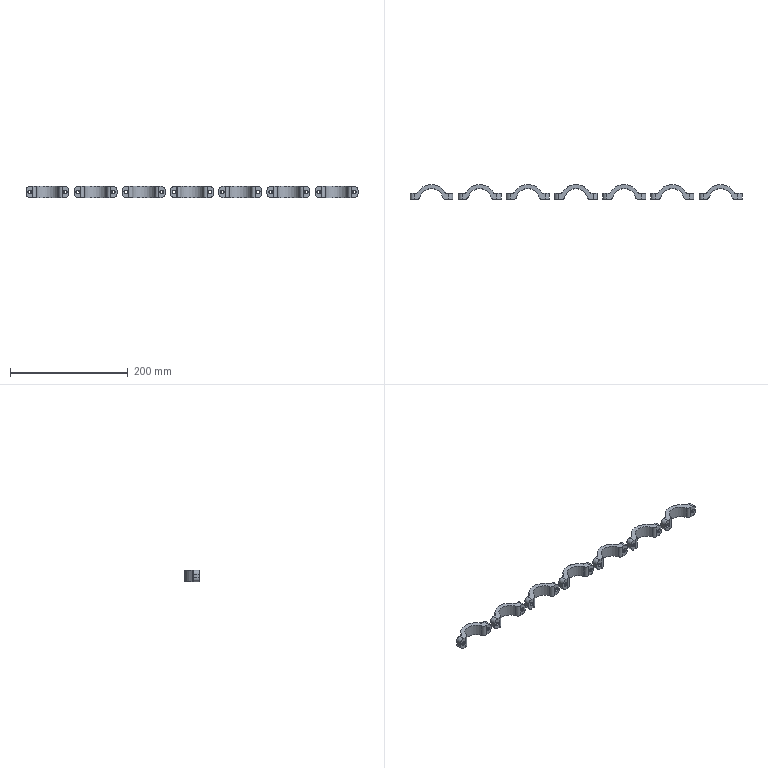NC program | Mastercam | posted with a generic post
Lines 1390 to 2922 of 23883:
(8 FI |TOOL - 2|DIA. OFF. - 2|LEN. - 2|TOOL DIA. - 8.)
N2848 T2 M6
N2850 G0 G56 G90 X28.858 Y7.56 C0. B0. S3500 M3
N2852 G43 H2 Z50.
N2854 Z1.
N2856 G1 Z-.5 F2000.
N2858 G41 D2 X24.866 Y4.549 F800.
N2860 G3 X24.786 Y4.389 I.121 J-.16
N2862 X24.827 Y4.269 I.201
N2864 G2 X26.441 Y1.912 I-24.827 J-18.731
N2866 G3 X26.714 Y1.475 I5.579 J3.182
N2868 X27.143 Y1.461 I.429 J6.407
N2870 X27.255 Y1.462 J6.421
N2872 G1 X31.884
N2874 G3 X32.084 Y1.662 J.2
N2876 G1 G40 Y6.662
N2878 X28.858 Y7.56
N2880 Z-1. F2000.
N2882 G41 D2 X24.866 Y4.549 F800.
N2884 G3 X24.786 Y4.389 I.121 J-.16
N2886 X24.827 Y4.269 I.201
N2888 G2 X26.441 Y1.912 I-24.827 J-18.731
N2890 G3 X26.714 Y1.475 I5.579 J3.182
N2892 X27.143 Y1.461 I.429 J6.407
N2894 X27.255 Y1.462 J6.421
N2896 G1 X31.884
N2898 G3 X32.084 Y1.662 J.2
N2900 G1 G40 Y6.662
N2902 X28.858 Y7.56
N2904 Z-1.5 F2000.
N2906 G41 D2 X24.866 Y4.549 F800.
N2908 G3 X24.786 Y4.389 I.121 J-.16
N2910 X24.827 Y4.269 I.201
N2912 G2 X26.441 Y1.912 I-24.827 J-18.731
N2914 G3 X26.714 Y1.475 I5.579 J3.182
N2916 X27.143 Y1.461 I.429 J6.407
N2918 X27.255 Y1.462 J6.421
N2920 G1 X31.884
N2922 G3 X32.084 Y1.662 J.2
N2924 G1 G40 Y6.662
N2926 X28.858 Y7.56
N2928 Z-2. F2000.
N2930 G41 D2 X24.866 Y4.549 F800.
N2932 G3 X24.786 Y4.389 I.121 J-.16
N2934 X24.827 Y4.269 I.201
N2936 G2 X26.441 Y1.912 I-24.827 J-18.731
N2938 G3 X26.714 Y1.475 I5.579 J3.182
N2940 X27.143 Y1.461 I.429 J6.407
N2942 X27.255 Y1.462 J6.421
N2944 G1 X31.884
N2946 G3 X32.084 Y1.662 J.2
N2948 G1 G40 Y6.662
N2950 X28.858 Y7.56
N2952 Z-2.5 F2000.
N2954 G41 D2 X24.866 Y4.549 F800.
N2956 G3 X24.786 Y4.389 I.121 J-.16
N2958 X24.827 Y4.269 I.201
N2960 G2 X26.441 Y1.912 I-24.827 J-18.731
N2962 G3 X26.714 Y1.475 I5.579 J3.182
N2964 X27.143 Y1.461 I.429 J6.407
N2966 X27.255 Y1.462 J6.421
N2968 G1 X31.884
N2970 G3 X32.084 Y1.662 J.2
N2972 G1 G40 Y6.662
N2974 X28.858 Y7.56
N2976 Z-3. F2000.
N2978 G41 D2 X24.866 Y4.549 F800.
N2980 G3 X24.786 Y4.389 I.121 J-.16
N2982 X24.827 Y4.269 I.201
N2984 G2 X26.441 Y1.912 I-24.827 J-18.731
N2986 G3 X26.714 Y1.475 I5.579 J3.182
N2988 X27.143 Y1.461 I.429 J6.407
N2990 X27.255 Y1.462 J6.421
N2992 G1 X31.884
N2994 G3 X32.084 Y1.662 J.2
N2996 G1 G40 Y6.662
N2998 X28.858 Y7.56
N3000 Z-3.5 F2000.
N3002 G41 D2 X24.866 Y4.549 F800.
N3004 G3 X24.786 Y4.389 I.121 J-.16
N3006 X24.827 Y4.269 I.201
N3008 G2 X26.441 Y1.912 I-24.827 J-18.731
N3010 G3 X26.714 Y1.475 I5.579 J3.182
N3012 X27.143 Y1.461 I.429 J6.407
N3014 X27.255 Y1.462 J6.421
N3016 G1 X31.884
N3018 G3 X32.084 Y1.662 J.2
N3020 G1 G40 Y6.662
N3022 X28.858 Y7.56
N3024 Z-4. F2000.
N3026 G41 D2 X24.866 Y4.549 F800.
N3028 G3 X24.786 Y4.389 I.121 J-.16
N3030 X24.827 Y4.269 I.201
N3032 G2 X26.441 Y1.912 I-24.827 J-18.731
N3034 G3 X26.714 Y1.475 I5.579 J3.182
N3036 X27.143 Y1.461 I.429 J6.407
N3038 X27.255 Y1.462 J6.421
N3040 G1 X31.884
N3042 G3 X32.084 Y1.662 J.2
N3044 G1 G40 Y6.662
N3046 X28.858 Y7.56
N3048 Z-4.5 F2000.
N3050 G41 D2 X24.866 Y4.549 F800.
N3052 G3 X24.786 Y4.389 I.121 J-.16
N3054 X24.827 Y4.269 I.201
N3056 G2 X26.441 Y1.912 I-24.827 J-18.731
N3058 G3 X26.714 Y1.475 I5.579 J3.182
N3060 X27.143 Y1.461 I.429 J6.407
N3062 X27.255 Y1.462 J6.421
N3064 G1 X31.884
N3066 G3 X32.084 Y1.662 J.2
N3068 G1 G40 Y6.662
N3070 X28.858 Y7.56
N3072 Z-5. F2000.
N3074 G41 D2 X24.866 Y4.549 F800.
N3076 G3 X24.786 Y4.389 I.121 J-.16
N3078 X24.827 Y4.269 I.201
N3080 G2 X26.441 Y1.912 I-24.827 J-18.731
N3082 G3 X26.714 Y1.475 I5.579 J3.182
N3084 X27.143 Y1.461 I.429 J6.407
N3086 X27.255 Y1.462 J6.421
N3088 G1 X31.884
N3090 G3 X32.084 Y1.662 J.2
N3092 G1 G40 Y6.662
N3094 X28.858 Y7.56
N3096 Z-5.5 F2000.
N3098 G41 D2 X24.866 Y4.549 F800.
N3100 G3 X24.786 Y4.389 I.121 J-.16
N3102 X24.827 Y4.269 I.201
N3104 G2 X26.441 Y1.912 I-24.827 J-18.731
N3106 G3 X26.714 Y1.475 I5.579 J3.182
N3108 X27.143 Y1.461 I.429 J6.407
N3110 X27.255 Y1.462 J6.421
N3112 G1 X31.884
N3114 G3 X32.084 Y1.662 J.2
N3116 G1 G40 Y6.662
N3118 X28.858 Y7.56
N3120 Z-6. F2000.
N3122 G41 D2 X24.866 Y4.549 F800.
N3124 G3 X24.786 Y4.389 I.121 J-.16
N3126 X24.827 Y4.269 I.201
N3128 G2 X26.441 Y1.912 I-24.827 J-18.731
N3130 G3 X26.714 Y1.475 I5.579 J3.182
N3132 X27.143 Y1.461 I.429 J6.407
N3134 X27.255 Y1.462 J6.421
N3136 G1 X31.884
N3138 G3 X32.084 Y1.662 J.2
N3140 G1 G40 Y6.662
N3142 X28.858 Y7.56
N3144 Z-6.5 F2000.
N3146 G41 D2 X24.866 Y4.549 F800.
N3148 G3 X24.786 Y4.389 I.121 J-.16
N3150 X24.827 Y4.269 I.201
N3152 G2 X26.441 Y1.912 I-24.827 J-18.731
N3154 G3 X26.714 Y1.475 I5.579 J3.182
N3156 X27.143 Y1.461 I.429 J6.407
N3158 X27.255 Y1.462 J6.421
N3160 G1 X31.884
N3162 G3 X32.084 Y1.662 J.2
N3164 G1 G40 Y6.662
N3166 X28.858 Y7.56
N3168 Z-7. F2000.
N3170 G41 D2 X24.866 Y4.549 F800.
N3172 G3 X24.786 Y4.389 I.121 J-.16
N3174 X24.827 Y4.269 I.201
N3176 G2 X26.441 Y1.912 I-24.827 J-18.731
N3178 G3 X26.714 Y1.475 I5.579 J3.182
N3180 X27.143 Y1.461 I.429 J6.407
N3182 X27.255 Y1.462 J6.421
N3184 G1 X31.884
N3186 G3 X32.084 Y1.662 J.2
N3188 G1 G40 Y6.662
N3190 X28.858 Y7.56
N3192 Z-7.5 F2000.
N3194 G41 D2 X24.866 Y4.549 F800.
N3196 G3 X24.786 Y4.389 I.121 J-.16
N3198 X24.827 Y4.269 I.201
N3200 G2 X26.441 Y1.912 I-24.827 J-18.731
N3202 G3 X26.714 Y1.475 I5.579 J3.182
N3204 X27.143 Y1.461 I.429 J6.407
N3206 X27.255 Y1.462 J6.421
N3208 G1 X31.884
N3210 G3 X32.084 Y1.662 J.2
N3212 G1 G40 Y6.662
N3214 X28.858 Y7.56
N3216 Z-8. F2000.
N3218 G41 D2 X24.866 Y4.549 F800.
N3220 G3 X24.786 Y4.389 I.121 J-.16
N3222 X24.827 Y4.269 I.201
N3224 G2 X26.441 Y1.912 I-24.827 J-18.731
N3226 G3 X26.714 Y1.475 I5.579 J3.182
N3228 X27.143 Y1.461 I.429 J6.407
N3230 X27.255 Y1.462 J6.421
N3232 G1 X31.884
N3234 G3 X32.084 Y1.662 J.2
N3236 G1 G40 Y6.662
N3238 X28.858 Y7.56
N3240 Z-8.5 F2000.
N3242 G41 D2 X24.866 Y4.549 F800.
N3244 G3 X24.786 Y4.389 I.121 J-.16
N3246 X24.827 Y4.269 I.201
N3248 G2 X26.441 Y1.912 I-24.827 J-18.731
N3250 G3 X26.714 Y1.475 I5.579 J3.182
N3252 X27.143 Y1.461 I.429 J6.407
N3254 X27.255 Y1.462 J6.421
N3256 G1 X31.884
N3258 G3 X32.084 Y1.662 J.2
N3260 G1 G40 Y6.662
N3262 X28.858 Y7.56
N3264 Z-9. F2000.
N3266 G41 D2 X24.866 Y4.549 F800.
N3268 G3 X24.786 Y4.389 I.121 J-.16
N3270 X24.827 Y4.269 I.201
N3272 G2 X26.441 Y1.912 I-24.827 J-18.731
N3274 G3 X26.714 Y1.475 I5.579 J3.182
N3276 X27.143 Y1.461 I.429 J6.407
N3278 X27.255 Y1.462 J6.421
N3280 G1 X31.884
N3282 G3 X32.084 Y1.662 J.2
N3284 G1 G40 Y6.662
N3286 X28.858 Y7.56
N3288 Z-9.5 F2000.
N3290 G41 D2 X24.866 Y4.549 F800.
N3292 G3 X24.786 Y4.389 I.121 J-.16
N3294 X24.827 Y4.269 I.201
N3296 G2 X26.441 Y1.912 I-24.827 J-18.731
N3298 G3 X26.714 Y1.475 I5.579 J3.182
N3300 X27.143 Y1.461 I.429 J6.407
N3302 X27.255 Y1.462 J6.421
N3304 G1 X31.884
N3306 G3 X32.084 Y1.662 J.2
N3308 G1 G40 Y6.662
N3310 X28.858 Y7.56
N3312 Z-10. F2000.
N3314 G41 D2 X24.866 Y4.549 F800.
N3316 G3 X24.786 Y4.389 I.121 J-.16
N3318 X24.827 Y4.269 I.201
N3320 G2 X26.441 Y1.912 I-24.827 J-18.731
N3322 G3 X26.714 Y1.475 I5.579 J3.182
N3324 X27.143 Y1.461 I.429 J6.407
N3326 X27.255 Y1.462 J6.421
N3328 G1 X31.884
N3330 G3 X32.084 Y1.662 J.2
N3332 G1 G40 Y6.662
N3334 X28.858 Y7.56
N3336 Z-10.5 F2000.
N3338 G41 D2 X24.866 Y4.549 F800.
N3340 G3 X24.786 Y4.389 I.121 J-.16
N3342 X24.827 Y4.269 I.201
N3344 G2 X26.441 Y1.912 I-24.827 J-18.731
N3346 G3 X26.714 Y1.475 I5.579 J3.182
N3348 X27.143 Y1.461 I.429 J6.407
N3350 X27.255 Y1.462 J6.421
N3352 G1 X31.884
N3354 G3 X32.084 Y1.662 J.2
N3356 G1 G40 Y6.662
N3358 X28.858 Y7.56
N3360 Z-11. F2000.
N3362 G41 D2 X24.866 Y4.549 F800.
N3364 G3 X24.786 Y4.389 I.121 J-.16
N3366 X24.827 Y4.269 I.201
N3368 G2 X26.441 Y1.912 I-24.827 J-18.731
N3370 G3 X26.714 Y1.475 I5.579 J3.182
N3372 X27.143 Y1.461 I.429 J6.407
N3374 X27.255 Y1.462 J6.421
N3376 G1 X31.884
N3378 G3 X32.084 Y1.662 J.2
N3380 G1 G40 Y6.662
N3382 X28.858 Y7.56
N3384 Z-11.5 F2000.
N3386 G41 D2 X24.866 Y4.549 F800.
N3388 G3 X24.786 Y4.389 I.121 J-.16
N3390 X24.827 Y4.269 I.201
N3392 G2 X26.441 Y1.912 I-24.827 J-18.731
N3394 G3 X26.714 Y1.475 I5.579 J3.182
N3396 X27.143 Y1.461 I.429 J6.407
N3398 X27.255 Y1.462 J6.421
N3400 G1 X31.884
N3402 G3 X32.084 Y1.662 J.2
N3404 G1 G40 Y6.662
N3406 X28.858 Y7.56
N3408 Z-12. F2000.
N3410 G41 D2 X24.866 Y4.549 F800.
N3412 G3 X24.786 Y4.389 I.121 J-.16
N3414 X24.827 Y4.269 I.201
N3416 G2 X26.441 Y1.912 I-24.827 J-18.731
N3418 G3 X26.714 Y1.475 I5.579 J3.182
N3420 X27.143 Y1.461 I.429 J6.407
N3422 X27.255 Y1.462 J6.421
N3424 G1 X31.884
N3426 G3 X32.084 Y1.662 J.2
N3428 G1 G40 Y6.662
N3430 X28.858 Y7.56
N3432 Z-12.5 F2000.
N3434 G41 D2 X24.866 Y4.549 F800.
N3436 G3 X24.786 Y4.389 I.121 J-.16
N3438 X24.827 Y4.269 I.201
N3440 G2 X26.441 Y1.912 I-24.827 J-18.731
N3442 G3 X26.714 Y1.475 I5.579 J3.182
N3444 X27.143 Y1.461 I.429 J6.407
N3446 X27.255 Y1.462 J6.421
N3448 G1 X31.884
N3450 G3 X32.084 Y1.662 J.2
N3452 G1 G40 Y6.662
N3454 X28.858 Y7.56
N3456 Z-13. F2000.
N3458 G41 D2 X24.866 Y4.549 F800.
N3460 G3 X24.786 Y4.389 I.121 J-.16
N3462 X24.827 Y4.269 I.201
N3464 G2 X26.441 Y1.912 I-24.827 J-18.731
N3466 G3 X26.714 Y1.475 I5.579 J3.182
N3468 X27.143 Y1.461 I.429 J6.407
N3470 X27.255 Y1.462 J6.421
N3472 G1 X31.884
N3474 G3 X32.084 Y1.662 J.2
N3476 G1 G40 Y6.662
N3478 X28.858 Y7.56
N3480 Z-13.5 F2000.
N3482 G41 D2 X24.866 Y4.549 F800.
N3484 G3 X24.786 Y4.389 I.121 J-.16
N3486 X24.827 Y4.269 I.201
N3488 G2 X26.441 Y1.912 I-24.827 J-18.731
N3490 G3 X26.714 Y1.475 I5.579 J3.182
N3492 X27.143 Y1.461 I.429 J6.407
N3494 X27.255 Y1.462 J6.421
N3496 G1 X31.884
N3498 G3 X32.084 Y1.662 J.2
N3500 G1 G40 Y6.662
N3502 X28.858 Y7.56
N3504 Z-14. F2000.
N3506 G41 D2 X24.866 Y4.549 F800.
N3508 G3 X24.786 Y4.389 I.121 J-.16
N3510 X24.827 Y4.269 I.201
N3512 G2 X26.441 Y1.912 I-24.827 J-18.731
N3514 G3 X26.714 Y1.475 I5.579 J3.182
N3516 X27.143 Y1.461 I.429 J6.407
N3518 X27.255 Y1.462 J6.421
N3520 G1 X31.884
N3522 G3 X32.084 Y1.662 J.2
N3524 G1 G40 Y6.662
N3526 X28.858 Y7.56
N3528 Z-14.5 F2000.
N3530 G41 D2 X24.866 Y4.549 F800.
N3532 G3 X24.786 Y4.389 I.121 J-.16
N3534 X24.827 Y4.269 I.201
N3536 G2 X26.441 Y1.912 I-24.827 J-18.731
N3538 G3 X26.714 Y1.475 I5.579 J3.182
N3540 X27.143 Y1.461 I.429 J6.407
N3542 X27.255 Y1.462 J6.421
N3544 G1 X31.884
N3546 G3 X32.084 Y1.662 J.2
N3548 G1 G40 Y6.662
N3550 X28.858 Y7.56
N3552 Z-15. F2000.
N3554 G41 D2 X24.866 Y4.549 F800.
N3556 G3 X24.786 Y4.389 I.121 J-.16
N3558 X24.827 Y4.269 I.201
N3560 G2 X26.441 Y1.912 I-24.827 J-18.731
N3562 G3 X26.714 Y1.475 I5.579 J3.182
N3564 X27.143 Y1.461 I.429 J6.407
N3566 X27.255 Y1.462 J6.421
N3568 G1 X31.884
N3570 G3 X32.084 Y1.662 J.2
N3572 G1 G40 Y6.662
N3574 X28.858 Y7.56
N3576 Z-15.5 F2000.
N3578 G41 D2 X24.866 Y4.549 F800.
N3580 G3 X24.786 Y4.389 I.121 J-.16
N3582 X24.827 Y4.269 I.201
N3584 G2 X26.441 Y1.912 I-24.827 J-18.731
N3586 G3 X26.714 Y1.475 I5.579 J3.182
N3588 X27.143 Y1.461 I.429 J6.407
N3590 X27.255 Y1.462 J6.421
N3592 G1 X31.884
N3594 G3 X32.084 Y1.662 J.2
N3596 G1 G40 Y6.662
N3598 X28.858 Y7.56
N3600 Z-16. F2000.
N3602 G41 D2 X24.866 Y4.549 F800.
N3604 G3 X24.786 Y4.389 I.121 J-.16
N3606 X24.827 Y4.269 I.201
N3608 G2 X26.441 Y1.912 I-24.827 J-18.731
N3610 G3 X26.714 Y1.475 I5.579 J3.182
N3612 X27.143 Y1.461 I.429 J6.407
N3614 X27.255 Y1.462 J6.421
N3616 G1 X31.884
N3618 G3 X32.084 Y1.662 J.2
N3620 G1 G40 Y6.662
N3622 X28.858 Y7.56
N3624 Z-16.5 F2000.
N3626 G41 D2 X24.866 Y4.549 F800.
N3628 G3 X24.786 Y4.389 I.121 J-.16
N3630 X24.827 Y4.269 I.201
N3632 G2 X26.441 Y1.912 I-24.827 J-18.731
N3634 G3 X26.714 Y1.475 I5.579 J3.182
N3636 X27.143 Y1.461 I.429 J6.407
N3638 X27.255 Y1.462 J6.421
N3640 G1 X31.884
N3642 G3 X32.084 Y1.662 J.2
N3644 G1 G40 Y6.662
N3646 X28.858 Y7.56
N3648 Z-17. F2000.
N3650 G41 D2 X24.866 Y4.549 F800.
N3652 G3 X24.786 Y4.389 I.121 J-.16
N3654 X24.827 Y4.269 I.201
N3656 G2 X26.441 Y1.912 I-24.827 J-18.731
N3658 G3 X26.714 Y1.475 I5.579 J3.182
N3660 X27.143 Y1.461 I.429 J6.407
N3662 X27.255 Y1.462 J6.421
N3664 G1 X31.884
N3666 G3 X32.084 Y1.662 J.2
N3668 G1 G40 Y6.662
N3670 X28.858 Y7.56
N3672 Z-17.5 F2000.
N3674 G41 D2 X24.866 Y4.549 F800.
N3676 G3 X24.786 Y4.389 I.121 J-.16
N3678 X24.827 Y4.269 I.201
N3680 G2 X26.441 Y1.912 I-24.827 J-18.731
N3682 G3 X26.714 Y1.475 I5.579 J3.182
N3684 X27.143 Y1.461 I.429 J6.407
N3686 X27.255 Y1.462 J6.421
N3688 G1 X31.884
N3690 G3 X32.084 Y1.662 J.2
N3692 G1 G40 Y6.662
N3694 X28.858 Y7.56
N3696 Z-18. F2000.
N3698 G41 D2 X24.866 Y4.549 F800.
N3700 G3 X24.786 Y4.389 I.121 J-.16
N3702 X24.827 Y4.269 I.201
N3704 G2 X26.441 Y1.912 I-24.827 J-18.731
N3706 G3 X26.714 Y1.475 I5.579 J3.182
N3708 X27.143 Y1.461 I.429 J6.407
N3710 X27.255 Y1.462 J6.421
N3712 G1 X31.884
N3714 G3 X32.084 Y1.662 J.2
N3716 G1 G40 Y6.662
N3718 X28.858 Y7.56
N3720 Z-18.5 F2000.
N3722 G41 D2 X24.866 Y4.549 F800.
N3724 G3 X24.786 Y4.389 I.121 J-.16
N3726 X24.827 Y4.269 I.201
N3728 G2 X26.441 Y1.912 I-24.827 J-18.731
N3730 G3 X26.714 Y1.475 I5.579 J3.182
N3732 X27.143 Y1.461 I.429 J6.407
N3734 X27.255 Y1.462 J6.421
N3736 G1 X31.884
N3738 G3 X32.084 Y1.662 J.2
N3740 G1 G40 Y6.662
N3742 X28.858 Y7.56
N3744 Z-19. F2000.
N3746 G41 D2 X24.866 Y4.549 F800.
N3748 G3 X24.786 Y4.389 I.121 J-.16
N3750 X24.827 Y4.269 I.201
N3752 G2 X26.441 Y1.912 I-24.827 J-18.731
N3754 G3 X26.714 Y1.475 I5.579 J3.182
N3756 X27.143 Y1.461 I.429 J6.407
N3758 X27.255 Y1.462 J6.421
N3760 G1 X31.884
N3762 G3 X32.084 Y1.662 J.2
N3764 G1 G40 Y6.662
N3766 X28.858 Y7.56
N3768 Z-19.5 F2000.
N3770 G41 D2 X24.866 Y4.549 F800.
N3772 G3 X24.786 Y4.389 I.121 J-.16
N3774 X24.827 Y4.269 I.201
N3776 G2 X26.441 Y1.912 I-24.827 J-18.731
N3778 G3 X26.714 Y1.475 I5.579 J3.182
N3780 X27.143 Y1.461 I.429 J6.407
N3782 X27.255 Y1.462 J6.421
N3784 G1 X31.884
N3786 G3 X32.084 Y1.662 J.2
N3788 G1 G40 Y6.662
N3790 X28.858 Y7.56
N3792 Z-20. F2000.
N3794 G41 D2 X24.866 Y4.549 F800.
N3796 G3 X24.786 Y4.389 I.121 J-.16
N3798 X24.827 Y4.269 I.201
N3800 G2 X26.441 Y1.912 I-24.827 J-18.731
N3802 G3 X26.714 Y1.475 I5.579 J3.182
N3804 X27.143 Y1.461 I.429 J6.407
N3806 X27.255 Y1.462 J6.421
N3808 G1 X31.884
N3810 G3 X32.084 Y1.662 J.2
N3812 G1 G40 Y6.662
N3814 X28.858 Y7.56
N3816 Z-20.5 F2000.
N3818 G41 D2 X24.866 Y4.549 F800.
N3820 G3 X24.786 Y4.389 I.121 J-.16
N3822 X24.827 Y4.269 I.201
N3824 G2 X26.441 Y1.912 I-24.827 J-18.731
N3826 G3 X26.714 Y1.475 I5.579 J3.182
N3828 X27.143 Y1.461 I.429 J6.407
N3830 X27.255 Y1.462 J6.421
N3832 G1 X31.884
N3834 G3 X32.084 Y1.662 J.2
N3836 G1 G40 Y6.662
N3838 X28.858 Y7.56
N3840 Z-21. F2000.
N3842 G41 D2 X24.866 Y4.549 F800.
N3844 G3 X24.786 Y4.389 I.121 J-.16
N3846 X24.827 Y4.269 I.201
N3848 G2 X26.441 Y1.912 I-24.827 J-18.731
N3850 G3 X26.714 Y1.475 I5.579 J3.182
N3852 X27.143 Y1.461 I.429 J6.407
N3854 X27.255 Y1.462 J6.421
N3856 G1 X31.884
N3858 G3 X32.084 Y1.662 J.2
N3860 G1 G40 Y6.662
N3862 G0 Z50.
N3864 X-32.052
N3866 Z1.
N3868 G1 Z-.5 F2000.
N3870 G41 D2 Y1.662 F800.
N3872 G3 X-31.852 Y1.462 I.2
N3874 G1 X-27.264
N3876 X-26.719 Y1.47
N3878 G2 X-24.827 Y4.269 I28.979 J-17.547
N3880 G3 X-24.787 Y4.389 I-.16 J.12
N3882 X-24.866 Y4.549 I-.2
N3884 G1 G40 X-28.858 Y7.56
N3886 X-32.052 Y6.662
N3888 Z-1. F2000.
N3890 G41 D2 Y1.662 F800.
N3892 G3 X-31.852 Y1.462 I.2
N3894 G1 X-27.264
N3896 X-26.719 Y1.47
N3898 G2 X-24.827 Y4.269 I28.979 J-17.547
N3900 G3 X-24.787 Y4.389 I-.16 J.12
N3902 X-24.866 Y4.549 I-.2
N3904 G1 G40 X-28.858 Y7.56
N3906 X-32.052 Y6.662
N3908 Z-1.5 F2000.
N3910 G41 D2 Y1.662 F800.
N3912 G3 X-31.852 Y1.462 I.2
N3914 G1 X-27.264
N3916 X-26.719 Y1.47
N3918 G2 X-24.827 Y4.269 I28.979 J-17.547
N3920 G3 X-24.787 Y4.389 I-.16 J.12
N3922 X-24.866 Y4.549 I-.2
N3924 G1 G40 X-28.858 Y7.56
N3926 X-32.052 Y6.662
N3928 Z-2. F2000.
N3930 G41 D2 Y1.662 F800.
N3932 G3 X-31.852 Y1.462 I.2
N3934 G1 X-27.264
N3936 X-26.719 Y1.47
N3938 G2 X-24.827 Y4.269 I28.979 J-17.547
N3940 G3 X-24.787 Y4.389 I-.16 J.12
N3942 X-24.866 Y4.549 I-.2
N3944 G1 G40 X-28.858 Y7.56
N3946 X-32.052 Y6.662
N3948 Z-2.5 F2000.
N3950 G41 D2 Y1.662 F800.
N3952 G3 X-31.852 Y1.462 I.2
N3954 G1 X-27.264
N3956 X-26.719 Y1.47
N3958 G2 X-24.827 Y4.269 I28.979 J-17.547
N3960 G3 X-24.787 Y4.389 I-.16 J.12
N3962 X-24.866 Y4.549 I-.2
N3964 G1 G40 X-28.858 Y7.56
N3966 X-32.052 Y6.662
N3968 Z-3. F2000.
N3970 G41 D2 Y1.662 F800.
N3972 G3 X-31.852 Y1.462 I.2
N3974 G1 X-27.264
N3976 X-26.719 Y1.47
N3978 G2 X-24.827 Y4.269 I28.979 J-17.547
N3980 G3 X-24.787 Y4.389 I-.16 J.12
N3982 X-24.866 Y4.549 I-.2
N3984 G1 G40 X-28.858 Y7.56
N3986 X-32.052 Y6.662
N3988 Z-3.5 F2000.
N3990 G41 D2 Y1.662 F800.
N3992 G3 X-31.852 Y1.462 I.2
N3994 G1 X-27.264
N3996 X-26.719 Y1.47
N3998 G2 X-24.827 Y4.269 I28.979 J-17.547
N4000 G3 X-24.787 Y4.389 I-.16 J.12
N4002 X-24.866 Y4.549 I-.2
N4004 G1 G40 X-28.858 Y7.56
N4006 X-32.052 Y6.662
N4008 Z-4. F2000.
N4010 G41 D2 Y1.662 F800.
N4012 G3 X-31.852 Y1.462 I.2
N4014 G1 X-27.264
N4016 X-26.719 Y1.47
N4018 G2 X-24.827 Y4.269 I28.979 J-17.547
N4020 G3 X-24.787 Y4.389 I-.16 J.12
N4022 X-24.866 Y4.549 I-.2
N4024 G1 G40 X-28.858 Y7.56
N4026 X-32.052 Y6.662
N4028 Z-4.5 F2000.
N4030 G41 D2 Y1.662 F800.
N4032 G3 X-31.852 Y1.462 I.2
N4034 G1 X-27.264
N4036 X-26.719 Y1.47
N4038 G2 X-24.827 Y4.269 I28.979 J-17.547
N4040 G3 X-24.787 Y4.389 I-.16 J.12
N4042 X-24.866 Y4.549 I-.2
N4044 G1 G40 X-28.858 Y7.56
N4046 X-32.052 Y6.662
N4048 Z-5. F2000.
N4050 G41 D2 Y1.662 F800.
N4052 G3 X-31.852 Y1.462 I.2
N4054 G1 X-27.264
N4056 X-26.719 Y1.47
N4058 G2 X-24.827 Y4.269 I28.979 J-17.547
N4060 G3 X-24.787 Y4.389 I-.16 J.12
N4062 X-24.866 Y4.549 I-.2
N4064 G1 G40 X-28.858 Y7.56
N4066 X-32.052 Y6.662
N4068 Z-5.5 F2000.
N4070 G41 D2 Y1.662 F800.
N4072 G3 X-31.852 Y1.462 I.2
N4074 G1 X-27.264
N4076 X-26.719 Y1.47
N4078 G2 X-24.827 Y4.269 I28.979 J-17.547
N4080 G3 X-24.787 Y4.389 I-.16 J.12
N4082 X-24.866 Y4.549 I-.2
N4084 G1 G40 X-28.858 Y7.56
N4086 X-32.052 Y6.662
N4088 Z-6. F2000.
N4090 G41 D2 Y1.662 F800.
N4092 G3 X-31.852 Y1.462 I.2
N4094 G1 X-27.264
N4096 X-26.719 Y1.47
N4098 G2 X-24.827 Y4.269 I28.979 J-17.547
N4100 G3 X-24.787 Y4.389 I-.16 J.12
N4102 X-24.866 Y4.549 I-.2
N4104 G1 G40 X-28.858 Y7.56
N4106 X-32.052 Y6.662
N4108 Z-6.5 F2000.
N4110 G41 D2 Y1.662 F800.
N4112 G3 X-31.852 Y1.462 I.2
N4114 G1 X-27.264
N4116 X-26.719 Y1.47
N4118 G2 X-24.827 Y4.269 I28.979 J-17.547
N4120 G3 X-24.787 Y4.389 I-.16 J.12
N4122 X-24.866 Y4.549 I-.2
N4124 G1 G40 X-28.858 Y7.56
N4126 X-32.052 Y6.662
N4128 Z-7. F2000.
N4130 G41 D2 Y1.662 F800.
N4132 G3 X-31.852 Y1.462 I.2
N4134 G1 X-27.264
N4136 X-26.719 Y1.47
N4138 G2 X-24.827 Y4.269 I28.979 J-17.547
N4140 G3 X-24.787 Y4.389 I-.16 J.12
N4142 X-24.866 Y4.549 I-.2
N4144 G1 G40 X-28.858 Y7.56
N4146 X-32.052 Y6.662
N4148 Z-7.5 F2000.
N4150 G41 D2 Y1.662 F800.
N4152 G3 X-31.852 Y1.462 I.2
N4154 G1 X-27.264
N4156 X-26.719 Y1.47
N4158 G2 X-24.827 Y4.269 I28.979 J-17.547
N4160 G3 X-24.787 Y4.389 I-.16 J.12
N4162 X-24.866 Y4.549 I-.2
N4164 G1 G40 X-28.858 Y7.56
N4166 X-32.052 Y6.662
N4168 Z-8. F2000.
N4170 G41 D2 Y1.662 F800.
N4172 G3 X-31.852 Y1.462 I.2
N4174 G1 X-27.264
N4176 X-26.719 Y1.47
N4178 G2 X-24.827 Y4.269 I28.979 J-17.547
N4180 G3 X-24.787 Y4.389 I-.16 J.12
N4182 X-24.866 Y4.549 I-.2
N4184 G1 G40 X-28.858 Y7.56
N4186 X-32.052 Y6.662
N4188 Z-8.5 F2000.
N4190 G41 D2 Y1.662 F800.
N4192 G3 X-31.852 Y1.462 I.2
N4194 G1 X-27.264
N4196 X-26.719 Y1.47
N4198 G2 X-24.827 Y4.269 I28.979 J-17.547
N4200 G3 X-24.787 Y4.389 I-.16 J.12
N4202 X-24.866 Y4.549 I-.2
N4204 G1 G40 X-28.858 Y7.56
N4206 X-32.052 Y6.662
N4208 Z-9. F2000.
N4210 G41 D2 Y1.662 F800.
N4212 G3 X-31.852 Y1.462 I.2
N4214 G1 X-27.264
N4216 X-26.719 Y1.47
N4218 G2 X-24.827 Y4.269 I28.979 J-17.547
N4220 G3 X-24.787 Y4.389 I-.16 J.12
N4222 X-24.866 Y4.549 I-.2
N4224 G1 G40 X-28.858 Y7.56
N4226 X-32.052 Y6.662
N4228 Z-9.5 F2000.
N4230 G41 D2 Y1.662 F800.
N4232 G3 X-31.852 Y1.462 I.2
N4234 G1 X-27.264
N4236 X-26.719 Y1.47
N4238 G2 X-24.827 Y4.269 I28.979 J-17.547
N4240 G3 X-24.787 Y4.389 I-.16 J.12
N4242 X-24.866 Y4.549 I-.2
N4244 G1 G40 X-28.858 Y7.56
N4246 X-32.052 Y6.662
N4248 Z-10. F2000.
N4250 G41 D2 Y1.662 F800.
N4252 G3 X-31.852 Y1.462 I.2
N4254 G1 X-27.264
N4256 X-26.719 Y1.47
N4258 G2 X-24.827 Y4.269 I28.979 J-17.547
N4260 G3 X-24.787 Y4.389 I-.16 J.12
N4262 X-24.866 Y4.549 I-.2
N4264 G1 G40 X-28.858 Y7.56
N4266 X-32.052 Y6.662
N4268 Z-10.5 F2000.
N4270 G41 D2 Y1.662 F800.
N4272 G3 X-31.852 Y1.462 I.2
N4274 G1 X-27.264
N4276 X-26.719 Y1.47
N4278 G2 X-24.827 Y4.269 I28.979 J-17.547
N4280 G3 X-24.787 Y4.389 I-.16 J.12
N4282 X-24.866 Y4.549 I-.2
N4284 G1 G40 X-28.858 Y7.56
N4286 X-32.052 Y6.662
N4288 Z-11. F2000.
N4290 G41 D2 Y1.662 F800.
N4292 G3 X-31.852 Y1.462 I.2
N4294 G1 X-27.264
N4296 X-26.719 Y1.47
N4298 G2 X-24.827 Y4.269 I28.979 J-17.547
N4300 G3 X-24.787 Y4.389 I-.16 J.12
N4302 X-24.866 Y4.549 I-.2
N4304 G1 G40 X-28.858 Y7.56
N4306 X-32.052 Y6.662
N4308 Z-11.5 F2000.
N4310 G41 D2 Y1.662 F800.
N4312 G3 X-31.852 Y1.462 I.2
N4314 G1 X-27.264
N4316 X-26.719 Y1.47
N4318 G2 X-24.827 Y4.269 I28.979 J-17.547
N4320 G3 X-24.787 Y4.389 I-.16 J.12
N4322 X-24.866 Y4.549 I-.2
N4324 G1 G40 X-28.858 Y7.56
N4326 X-32.052 Y6.662
N4328 Z-12. F2000.
N4330 G41 D2 Y1.662 F800.
N4332 G3 X-31.852 Y1.462 I.2
N4334 G1 X-27.264
N4336 X-26.719 Y1.47
N4338 G2 X-24.827 Y4.269 I28.979 J-17.547
N4340 G3 X-24.787 Y4.389 I-.16 J.12
N4342 X-24.866 Y4.549 I-.2
N4344 G1 G40 X-28.858 Y7.56
N4346 X-32.052 Y6.662
N4348 Z-12.5 F2000.
N4350 G41 D2 Y1.662 F800.
N4352 G3 X-31.852 Y1.462 I.2
N4354 G1 X-27.264
N4356 X-26.719 Y1.47
N4358 G2 X-24.827 Y4.269 I28.979 J-17.547
N4360 G3 X-24.787 Y4.389 I-.16 J.12
N4362 X-24.866 Y4.549 I-.2
N4364 G1 G40 X-28.858 Y7.56
N4366 X-32.052 Y6.662
N4368 Z-13. F2000.
N4370 G41 D2 Y1.662 F800.
N4372 G3 X-31.852 Y1.462 I.2
N4374 G1 X-27.264
N4376 X-26.719 Y1.47
N4378 G2 X-24.827 Y4.269 I28.979 J-17.547
N4380 G3 X-24.787 Y4.389 I-.16 J.12
N4382 X-24.866 Y4.549 I-.2
N4384 G1 G40 X-28.858 Y7.56
N4386 X-32.052 Y6.662
N4388 Z-13.5 F2000.
N4390 G41 D2 Y1.662 F800.
N4392 G3 X-31.852 Y1.462 I.2
N4394 G1 X-27.264
N4396 X-26.719 Y1.47
N4398 G2 X-24.827 Y4.269 I28.979 J-17.547
N4400 G3 X-24.787 Y4.389 I-.16 J.12
N4402 X-24.866 Y4.549 I-.2
N4404 G1 G40 X-28.858 Y7.56
N4406 X-32.052 Y6.662
N4408 Z-14. F2000.
N4410 G41 D2 Y1.662 F800.
N4412 G3 X-31.852 Y1.462 I.2
N4414 G1 X-27.264
N4416 X-26.719 Y1.47
N4418 G2 X-24.827 Y4.269 I28.979 J-17.547
N4420 G3 X-24.787 Y4.389 I-.16 J.12
N4422 X-24.866 Y4.549 I-.2
N4424 G1 G40 X-28.858 Y7.56
N4426 X-32.052 Y6.662
N4428 Z-14.5 F2000.
N4430 G41 D2 Y1.662 F800.
N4432 G3 X-31.852 Y1.462 I.2
N4434 G1 X-27.264
N4436 X-26.719 Y1.47
N4438 G2 X-24.827 Y4.269 I28.979 J-17.547
N4440 G3 X-24.787 Y4.389 I-.16 J.12
N4442 X-24.866 Y4.549 I-.2
N4444 G1 G40 X-28.858 Y7.56
N4446 X-32.052 Y6.662
N4448 Z-15. F2000.
N4450 G41 D2 Y1.662 F800.
N4452 G3 X-31.852 Y1.462 I.2
N4454 G1 X-27.264
N4456 X-26.719 Y1.47
N4458 G2 X-24.827 Y4.269 I28.979 J-17.547
N4460 G3 X-24.787 Y4.389 I-.16 J.12
N4462 X-24.866 Y4.549 I-.2
N4464 G1 G40 X-28.858 Y7.56
N4466 X-32.052 Y6.662
N4468 Z-15.5 F2000.
N4470 G41 D2 Y1.662 F800.
N4472 G3 X-31.852 Y1.462 I.2
N4474 G1 X-27.264
N4476 X-26.719 Y1.47
N4478 G2 X-24.827 Y4.269 I28.979 J-17.547
N4480 G3 X-24.787 Y4.389 I-.16 J.12
N4482 X-24.866 Y4.549 I-.2
N4484 G1 G40 X-28.858 Y7.56
N4486 X-32.052 Y6.662
N4488 Z-16. F2000.
N4490 G41 D2 Y1.662 F800.
N4492 G3 X-31.852 Y1.462 I.2
N4494 G1 X-27.264
N4496 X-26.719 Y1.47
N4498 G2 X-24.827 Y4.269 I28.979 J-17.547
N4500 G3 X-24.787 Y4.389 I-.16 J.12
N4502 X-24.866 Y4.549 I-.2
N4504 G1 G40 X-28.858 Y7.56
N4506 X-32.052 Y6.662
N4508 Z-16.5 F2000.
N4510 G41 D2 Y1.662 F800.
N4512 G3 X-31.852 Y1.462 I.2
N4514 G1 X-27.264
N4516 X-26.719 Y1.47
N4518 G2 X-24.827 Y4.269 I28.979 J-17.547
N4520 G3 X-24.787 Y4.389 I-.16 J.12
N4522 X-24.866 Y4.549 I-.2
N4524 G1 G40 X-28.858 Y7.56
N4526 X-32.052 Y6.662
N4528 Z-17. F2000.
N4530 G41 D2 Y1.662 F800.
N4532 G3 X-31.852 Y1.462 I.2
N4534 G1 X-27.264
N4536 X-26.719 Y1.47
N4538 G2 X-24.827 Y4.269 I28.979 J-17.547
N4540 G3 X-24.787 Y4.389 I-.16 J.12
N4542 X-24.866 Y4.549 I-.2
N4544 G1 G40 X-28.858 Y7.56
N4546 X-32.052 Y6.662
N4548 Z-17.5 F2000.
N4550 G41 D2 Y1.662 F800.
N4552 G3 X-31.852 Y1.462 I.2
N4554 G1 X-27.264
N4556 X-26.719 Y1.47
N4558 G2 X-24.827 Y4.269 I28.979 J-17.547
N4560 G3 X-24.787 Y4.389 I-.16 J.12
N4562 X-24.866 Y4.549 I-.2
N4564 G1 G40 X-28.858 Y7.56
N4566 X-32.052 Y6.662
N4568 Z-18. F2000.
N4570 G41 D2 Y1.662 F800.
N4572 G3 X-31.852 Y1.462 I.2
N4574 G1 X-27.264
N4576 X-26.719 Y1.47
N4578 G2 X-24.827 Y4.269 I28.979 J-17.547
N4580 G3 X-24.787 Y4.389 I-.16 J.12
N4582 X-24.866 Y4.549 I-.2
N4584 G1 G40 X-28.858 Y7.56
N4586 X-32.052 Y6.662
N4588 Z-18.5 F2000.
N4590 G41 D2 Y1.662 F800.
N4592 G3 X-31.852 Y1.462 I.2
N4594 G1 X-27.264
N4596 X-26.719 Y1.47
N4598 G2 X-24.827 Y4.269 I28.979 J-17.547
N4600 G3 X-24.787 Y4.389 I-.16 J.12
N4602 X-24.866 Y4.549 I-.2
N4604 G1 G40 X-28.858 Y7.56
N4606 X-32.052 Y6.662
N4608 Z-19. F2000.
N4610 G41 D2 Y1.662 F800.
N4612 G3 X-31.852 Y1.462 I.2
N4614 G1 X-27.264
N4616 X-26.719 Y1.47
N4618 G2 X-24.827 Y4.269 I28.979 J-17.547
N4620 G3 X-24.787 Y4.389 I-.16 J.12
N4622 X-24.866 Y4.549 I-.2
N4624 G1 G40 X-28.858 Y7.56
N4626 X-32.052 Y6.662
N4628 Z-19.5 F2000.
N4630 G41 D2 Y1.662 F800.
N4632 G3 X-31.852 Y1.462 I.2
N4634 G1 X-27.264
N4636 X-26.719 Y1.47
N4638 G2 X-24.827 Y4.269 I28.979 J-17.547
N4640 G3 X-24.787 Y4.389 I-.16 J.12
N4642 X-24.866 Y4.549 I-.2
N4644 G1 G40 X-28.858 Y7.56
N4646 X-32.052 Y6.662
N4648 Z-20. F2000.
N4650 G41 D2 Y1.662 F800.
N4652 G3 X-31.852 Y1.462 I.2
N4654 G1 X-27.264
N4656 X-26.719 Y1.47
N4658 G2 X-24.827 Y4.269 I28.979 J-17.547
N4660 G3 X-24.787 Y4.389 I-.16 J.12
N4662 X-24.866 Y4.549 I-.2
N4664 G1 G40 X-28.858 Y7.56
N4666 X-32.052 Y6.662
N4668 Z-20.5 F2000.
N4670 G41 D2 Y1.662 F800.
N4672 G3 X-31.852 Y1.462 I.2
N4674 G1 X-27.264
N4676 X-26.719 Y1.47
N4678 G2 X-24.827 Y4.269 I28.979 J-17.547
N4680 G3 X-24.787 Y4.389 I-.16 J.12
N4682 X-24.866 Y4.549 I-.2
N4684 G1 G40 X-28.858 Y7.56
N4686 X-32.052 Y6.662
N4688 Z-21. F2000.
N4690 G41 D2 Y1.662 F800.
N4692 G3 X-31.852 Y1.462 I.2
N4694 G1 X-27.264
N4696 X-26.719 Y1.47
N4698 G2 X-24.827 Y4.269 I28.979 J-17.547
N4700 G3 X-24.787 Y4.389 I-.16 J.12
N4702 X-24.866 Y4.549 I-.2
N4704 G1 G40 X-28.858 Y7.56
N4706 G0 Z50.
N4708 X-20.553 Y-16.588
N4710 Z1.
N4712 G1 Z-21. F2000.
N4714 G41 D2 X-25.553 F800.
N4716 X-36.
N4718 G2 X-38.828 Y-15.417 J4.
N4720 G1 X-39.328 Y-14.917
N4722 G2 X-40.5 Y-12.088 I2.828 J2.829
N4724 G1 Y-3.088
N4726 G2 X-39.328 Y-.26 I4.
N4728 G1 X-38.828 Y.24
N4730 G2 X-36. Y1.412 I2.828 J-2.828
N4732 G1 X-27.264
N4734 G3 X-27.091 Y1.41 I.173 J6.585
N4736 X-26.69 Y1.421 J6.587
N4738 G2 X0. Y16.589 I26.69 J-15.899
N4740 X26.687 Y1.426 J-31.067
N4742 G3 X27.144 Y1.41 I.457 J6.729
N4744 X27.255 Y1.412 J6.745
N4746 G1 X36.
N4748 G2 X38.828 Y.24 J-4.
N4750 G1 X39.328 Y-.26
N4752 G2 X40.5 Y-3.088 I-2.828 J-2.828
N4754 G1 Y-12.088
N4756 G2 X39.328 Y-14.917 I-4.
N4758 G1 X38.828 Y-15.417
N4760 G2 X36. Y-16.588 I-2.828 J2.829
N4762 G1 X25.553
N4764 G40 X20.553
N4766 G0 Z50.
N4768 M5
N4770 G0 G28 G91 Z0.
N4772 G28
N4774 M01
N4776 G0 G17 G40 G80 G90 G94 G98
N4778 G0 G28 G91 Z0.
(6R0.5 MI |TOOL - 3|DIA. OFF. - 3|LEN. - 3|TOOL DIA. - 6.)
N4780 T3 M6
N4782 G0 G56 G90 X39.5 Y.412 C0. B0. S6500 M3
N4784 G43 H3 Z42.5
N4786 Z-2.5
N4788 G1 Z-7.5 F600.
N4790 Y-2.588 F4000.
N4792 Y-12.588
N4794 Y-15.588
N4796 Z-7.278
N4798 X39.497
N4800 Y-12.588
N4802 Y-2.588
N4804 Y.412
N4806 Z-7.053
N4808 X39.487
N4810 Y-2.588
N4812 Y-12.588
N4814 Y-15.588
N4816 Z-6.826
N4818 X39.47
N4820 Y-12.588
N4822 Y-2.588
N4824 Y.412
N4826 Z-6.597
N4828 X39.445
N4830 Y-2.588
N4832 Y-12.588
N4834 Y-15.588
N4836 Z-6.367
N4838 X39.414
N4840 Y-12.588
N4842 Y-2.588
N4844 Y.412
N4846 Z-6.135
N4848 X39.375
N4850 Y-2.588
N4852 Y-12.588
N4854 Y-15.588
N4856 Z-5.903
N4858 X39.328
N4860 Y-12.588
N4862 Y-2.588
N4864 Y.412
N4866 Z-5.67
N4868 X39.273
N4870 Y-2.588
N4872 Y-12.588
N4874 Y-15.588
N4876 Z-5.436
N4878 X39.21
N4880 Y-12.588
N4882 Y-2.588
N4884 Y.412
N4886 Z-5.203
N4888 X39.14
N4890 Y-2.588
N4892 Y-12.588
N4894 Y-15.588
N4896 Z-4.971
N4898 X39.061
N4900 Y-12.588
N4902 Y-2.588
N4904 Y.412
N4906 Z-4.739
N4908 X38.973
N4910 Y-2.588
N4912 Y-12.588
N4914 Y-15.588
N4916 Z-4.509
N4918 X38.878
N4920 Y-12.588
N4922 Y-2.588
N4924 Y.412
N4926 Z-4.281
N4928 X38.774
N4930 Y-2.588
N4932 Y-12.588
N4934 Y-15.588
N4936 Z-4.055
N4938 X38.662
N4940 Y-12.588
N4942 Y-2.588
N4944 Y.412
N4946 Z-3.832
N4948 X38.542
N4950 Y-2.588
N4952 Y-12.588
N4954 Y-15.588
N4956 Z-3.612
N4958 X38.414
N4960 Y-12.588
N4962 Y-2.588
N4964 Y.412
N4966 Z-3.396
N4968 X38.277
N4970 Y-2.588
N4972 Y-12.588
N4974 Y-15.588
N4976 Z-3.184
N4978 X38.133
N4980 Y-12.588
N4982 Y-2.588
N4984 Y.412
N4986 Z-2.976
N4988 X37.982
N4990 Y-2.588
N4992 Y-12.588
N4994 Y-15.588
N4996 Z-2.773
N4998 X37.823
N5000 Y-12.588
N5002 Y-2.588
N5004 Y.412
N5006 Z-2.575
N5008 X37.656
N5010 Y-2.588
N5012 Y-12.588
N5014 Y-15.588
N5016 Z-2.383
N5018 X37.483
N5020 Y-12.588
N5022 Y-2.588
N5024 Y.412
N5026 Z-2.197
N5028 X37.303
N5030 Y-2.588
N5032 Y-12.588
N5034 Y-15.588
N5036 Z-2.017
N5038 X37.117
N5040 Y-12.588
N5042 Y-2.588
N5044 Y.412
N5046 Z-1.844
N5048 X36.925
N5050 Y-2.588
N5052 Y-12.588
N5054 Y-15.588
N5056 Z-1.677
N5058 X36.727
N5060 Y-12.588
N5062 Y-2.588
N5064 Y.412
N5066 Z-1.518
N5068 X36.524
N5070 Y-2.588
N5072 Y-12.588
N5074 Y-15.588
N5076 Z-1.367
N5078 X36.316
N5080 Y-12.588
N5082 Y-2.588
N5084 Y.412
N5086 Z-1.223
N5088 X36.104
N5090 Y-2.588
N5092 Y-12.588
N5094 Y-15.588
N5096 Z-1.086
N5098 X35.888
N5100 Y-12.588
N5102 Y-2.588
N5104 Y.412
N5106 Z-.958
N5108 X35.668
N5110 Y-2.588
N5112 Y-12.588
N5114 Y-15.588
N5116 Z-.838
N5118 X35.445
N5120 Y-12.588
N5122 Y-2.588
N5124 Y.412
N5126 Z-.726
N5128 X35.219
N5130 Y-2.588
N5132 Y-12.588
N5134 Y-15.588
N5136 Z-.622
N5138 X34.991
N5140 Y-12.588
N5142 Y-2.588
N5144 Y.412
N5146 Z-.527
N5148 X34.761
N5150 Y-2.588
N5152 Y-12.588
N5154 Y-15.588
N5156 Z-.439
N5158 X34.529
N5160 Y-12.588
N5162 Y-2.588
N5164 Y.412
N5166 Z-.36
N5168 X34.297
N5170 Y-2.588
N5172 Y-12.588
N5174 Y-15.588
N5176 Z-.29
N5178 X34.064
N5180 Y-12.588
N5182 Y-2.588
N5184 Y.412
N5186 Z-.227
N5188 X33.83
N5190 Y-2.588
N5192 Y-12.588
N5194 Y-15.588
N5196 Z-.172
N5198 X33.597
N5200 Y-12.588
N5202 Y-2.588
N5204 Y.412
N5206 Z-.125
N5208 X33.365
N5210 Y-2.588
N5212 Y-12.588
N5214 Y-15.588
N5216 Z-.086
N5218 X33.133
N5220 Y-12.588
N5222 Y-2.588
N5224 Y.412
N5226 Z-.055
N5228 X32.903
N5230 Y-2.588
N5232 Y-12.588
N5234 Y-15.588
N5236 Z-.03
N5238 X32.674
N5240 Y-12.588
N5242 Y-2.588
N5244 Y.412
N5246 Z-.013
N5248 X32.447
N5250 Y-2.588
N5252 Y-12.588
N5254 Y-15.588
N5256 Z-.003
N5258 X32.222
N5260 Y-12.588
N5262 Y-2.588
N5264 Y.412
N5266 Z0.
N5268 X32.
N5270 Y-2.588
N5272 Y-12.588
N5274 Y-15.588
N5276 G0 Z5.
N5278 Z50.
N5280 X-39.5
N5282 Z42.5
N5284 Z-2.5
N5286 G1 Z-7.5 F600.
N5288 Y-12.588 F4000.
N5290 Y-2.588
N5292 Y.412
N5294 Z-7.278
N5296 X-39.497
N5298 Y-2.588
N5300 Y-12.588
N5302 Y-15.588
N5304 Z-7.053
N5306 X-39.487
N5308 Y-12.588
N5310 Y-2.588
N5312 Y.412
N5314 Z-6.826
N5316 X-39.47
N5318 Y-2.588
N5320 Y-12.588
N5322 Y-15.588
N5324 Z-6.597
N5326 X-39.445
N5328 Y-12.588
N5330 Y-2.588
N5332 Y.412
N5334 Z-6.367
N5336 X-39.414
N5338 Y-2.588
N5340 Y-12.588
N5342 Y-15.588
N5344 Z-6.135
N5346 X-39.375
N5348 Y-12.588
N5350 Y-2.588
N5352 Y.412
N5354 Z-5.903
N5356 X-39.328
N5358 Y-2.588
N5360 Y-12.588
N5362 Y-15.588
N5364 Z-5.67
N5366 X-39.273
N5368 Y-12.588
N5370 Y-2.588
N5372 Y.412
N5374 Z-5.436
N5376 X-39.21
N5378 Y-2.588
N5380 Y-12.588
N5382 Y-15.588
N5384 Z-5.203
N5386 X-39.14
N5388 Y-12.588
N5390 Y-2.588
N5392 Y.412
N5394 Z-4.971
N5396 X-39.061
N5398 Y-2.588
N5400 Y-12.588
N5402 Y-15.588
N5404 Z-4.739
N5406 X-38.973
N5408 Y-12.588
N5410 Y-2.588
N5412 Y.412
N5414 Z-4.509
N5416 X-38.878
N5418 Y-2.588
N5420 Y-12.588
N5422 Y-15.588
N5424 Z-4.281
N5426 X-38.774
N5428 Y-12.588
N5430 Y-2.588
N5432 Y.412
N5434 Z-4.055
N5436 X-38.662
N5438 Y-2.588
N5440 Y-12.588
N5442 Y-15.588
N5444 Z-3.832
N5446 X-38.542
N5448 Y-12.588
N5450 Y-2.588
N5452 Y.412
N5454 Z-3.612
N5456 X-38.414
N5458 Y-2.588
N5460 Y-12.588
N5462 Y-15.588
N5464 Z-3.396
N5466 X-38.277
N5468 Y-12.588
N5470 Y-2.588
N5472 Y.412
N5474 Z-3.184
N5476 X-38.133
N5478 Y-2.588
N5480 Y-12.588
N5482 Y-15.588
N5484 Z-2.976
N5486 X-37.982
N5488 Y-12.588
N5490 Y-2.588
N5492 Y.412
N5494 Z-2.773
N5496 X-37.823
N5498 Y-2.588
N5500 Y-12.588
N5502 Y-15.588
N5504 Z-2.575
N5506 X-37.656
N5508 Y-12.588
N5510 Y-2.588
N5512 Y.412
N5514 Z-2.383
N5516 X-37.483
N5518 Y-2.588
N5520 Y-12.588
N5522 Y-15.588
N5524 Z-2.197
N5526 X-37.303
N5528 Y-12.588
N5530 Y-2.588
N5532 Y.412
N5534 Z-2.017
N5536 X-37.117
N5538 Y-2.588
N5540 Y-12.588
N5542 Y-15.588
N5544 Z-1.844
N5546 X-36.925
N5548 Y-12.588
N5550 Y-2.588
N5552 Y.412
N5554 Z-1.677
N5556 X-36.727
N5558 Y-2.588
N5560 Y-12.588
N5562 Y-15.588
N5564 Z-1.518
N5566 X-36.524
N5568 Y-12.588
N5570 Y-2.588
N5572 Y.412
N5574 Z-1.367
N5576 X-36.316
N5578 Y-2.588
N5580 Y-12.588
N5582 Y-15.588
N5584 Z-1.223
N5586 X-36.104
N5588 Y-12.588
N5590 Y-2.588
N5592 Y.412
N5594 Z-1.086
N5596 X-35.888
N5598 Y-2.588
N5600 Y-12.588
N5602 Y-15.588
N5604 Z-.958
N5606 X-35.668
N5608 Y-12.588
N5610 Y-2.588
N5612 Y.412
N5614 Z-.838
N5616 X-35.445
N5618 Y-2.588
N5620 Y-12.588
N5622 Y-15.588
N5624 Z-.726
N5626 X-35.219
N5628 Y-12.588
N5630 Y-2.588
N5632 Y.412
N5634 Z-.622
N5636 X-34.991
N5638 Y-2.588
N5640 Y-12.588
N5642 Y-15.588
N5644 Z-.527
N5646 X-34.761
N5648 Y-12.588
N5650 Y-2.588
N5652 Y.412
N5654 Z-.439
N5656 X-34.529
N5658 Y-2.588
N5660 Y-12.588
N5662 Y-15.588
N5664 Z-.36
N5666 X-34.297
N5668 Y-12.588
N5670 Y-2.588
N5672 Y.412
N5674 Z-.29
N5676 X-34.064
N5678 Y-2.588
N5680 Y-12.588
N5682 Y-15.588
N5684 Z-.227
N5686 X-33.83
N5688 Y-12.588
N5690 Y-2.588
N5692 Y.412
N5694 Z-.172
N5696 X-33.597
N5698 Y-2.588
N5700 Y-12.588
N5702 Y-15.588
N5704 Z-.125
N5706 X-33.365
N5708 Y-12.588
N5710 Y-2.588
N5712 Y.412
N5714 Z-.086
N5716 X-33.133
N5718 Y-2.588
N5720 Y-12.588
N5722 Y-15.588
N5724 Z-.055
N5726 X-32.903
N5728 Y-12.588
N5730 Y-2.588
N5732 Y.412
N5734 Z-.03
N5736 X-32.674
N5738 Y-2.588
N5740 Y-12.588
N5742 Y-15.588
N5744 Z-.013
N5746 X-32.447
N5748 Y-12.588
N5750 Y-2.588
N5752 Y.412
N5754 Z-.003
N5756 X-32.222
N5758 Y-2.588
N5760 Y-12.588
N5762 Y-15.588
N5764 Z0.
N5766 X-32.
N5768 Y-12.588
N5770 Y-2.588
N5772 Y.412
N5774 G0 Z5.
N5776 Z50.
N5778 M5
N5780 G0 G28 G91 Z0.
N5782 G28
N5784 M01
N5786 G0 G17 G40 G80 G90 G94 G98
N5788 G0 G28 G91 Z0.
(6 CHM |TOOL - 4|DIA. OFF. - 4|LEN. - 4|TOOL DIA. - 6.)
N5790 T4 M6
N5792 G0 G56 G90 X-39. Y-1.588 C0. B0. S5000 M3
N5794 G43 H4 Z50.
N5796 Z1.
N5798 G1 Z-1.3 F2000.
N5800 G41 D4 X-36. F1000.
N5802 X-27.253
N5804 G3 X-27.066 Y-1.59 I.187 J9.295
N5806 X-25.929 Y-1.521 J9.297
N5808 X-24.57 Y-.761 I-.277 J2.091
N5810 X-23.846 Y.308 I-6.424 J5.126
N5812 G2 X.003 Y13.59 I23.849 J-14.771
N5814 X24.129 Y-.148 J-28.053
N5816 G3 X24.727 Y-.932 I3.792 J2.268
N5818 X25.72 Y-1.477 I1.426 J1.424
N5820 X26.8 Y-1.589 I1.08 J5.163
N5822 X26.916 Y-1.587 J5.275
N5824 G1 X27.251 Y-1.588
N5826 X36.
N5828 G40 X39.
N5830 G0 Z50.
N5832 Y-13.588
N5834 Z1.
N5836 G1 Z-1.3 F2000.
N5838 G41 D4 X36. F1000.
N5840 X25.549
N5842 G2 X25.237 Y-13.59 I-.312 J23.193
N5844 X23.783 Y-13.545 J23.195
N5846 G1 X22.861 Y-13.437
N5848 G2 X21.928 Y-13.215 I1.174 J7.023
N5850 G1 X21.157 Y-12.908
N5852 X20.478 Y-12.501
N5854 X19.893 Y-12.001
N5856 X19.393 Y-11.409
N5858 X18.966 Y-10.721
N5860 X18.592 Y-9.912
N5862 G2 X17.994 Y-8.208 I39.077 J14.666
N5864 G3 X0. Y4.588 I-17.994 J-6.254
N5866 X-17.995 Y-8.211 J-19.05
N5868 G1 X-18.457 Y-9.561
N5870 G2 X-19.029 Y-10.834 I-7.993 J2.826
N5872 G1 X-19.267 Y-11.226
N5874 X-19.764 Y-11.867
N5876 X-20.338 Y-12.396
N5878 X-20.98 Y-12.816
N5880 X-21.694 Y-13.137
N5882 X-22.489 Y-13.365
N5884 X-23.388 Y-13.51
N5886 G2 X-25.198 Y-13.592 I-1.81 J19.936
N5888 X-25.548 Y-13.588 J20.018
N5890 G1 X-36.
N5892 G40 X-39.
N5894 G0 Z50.
N5896 M5
N5898 G0 G28 G91 Z0.
N5900 G28
N5902 M01
N5904 G0 G17 G40 G80 G90 G94 G98
N5906 G0 G28 G91 Z0.